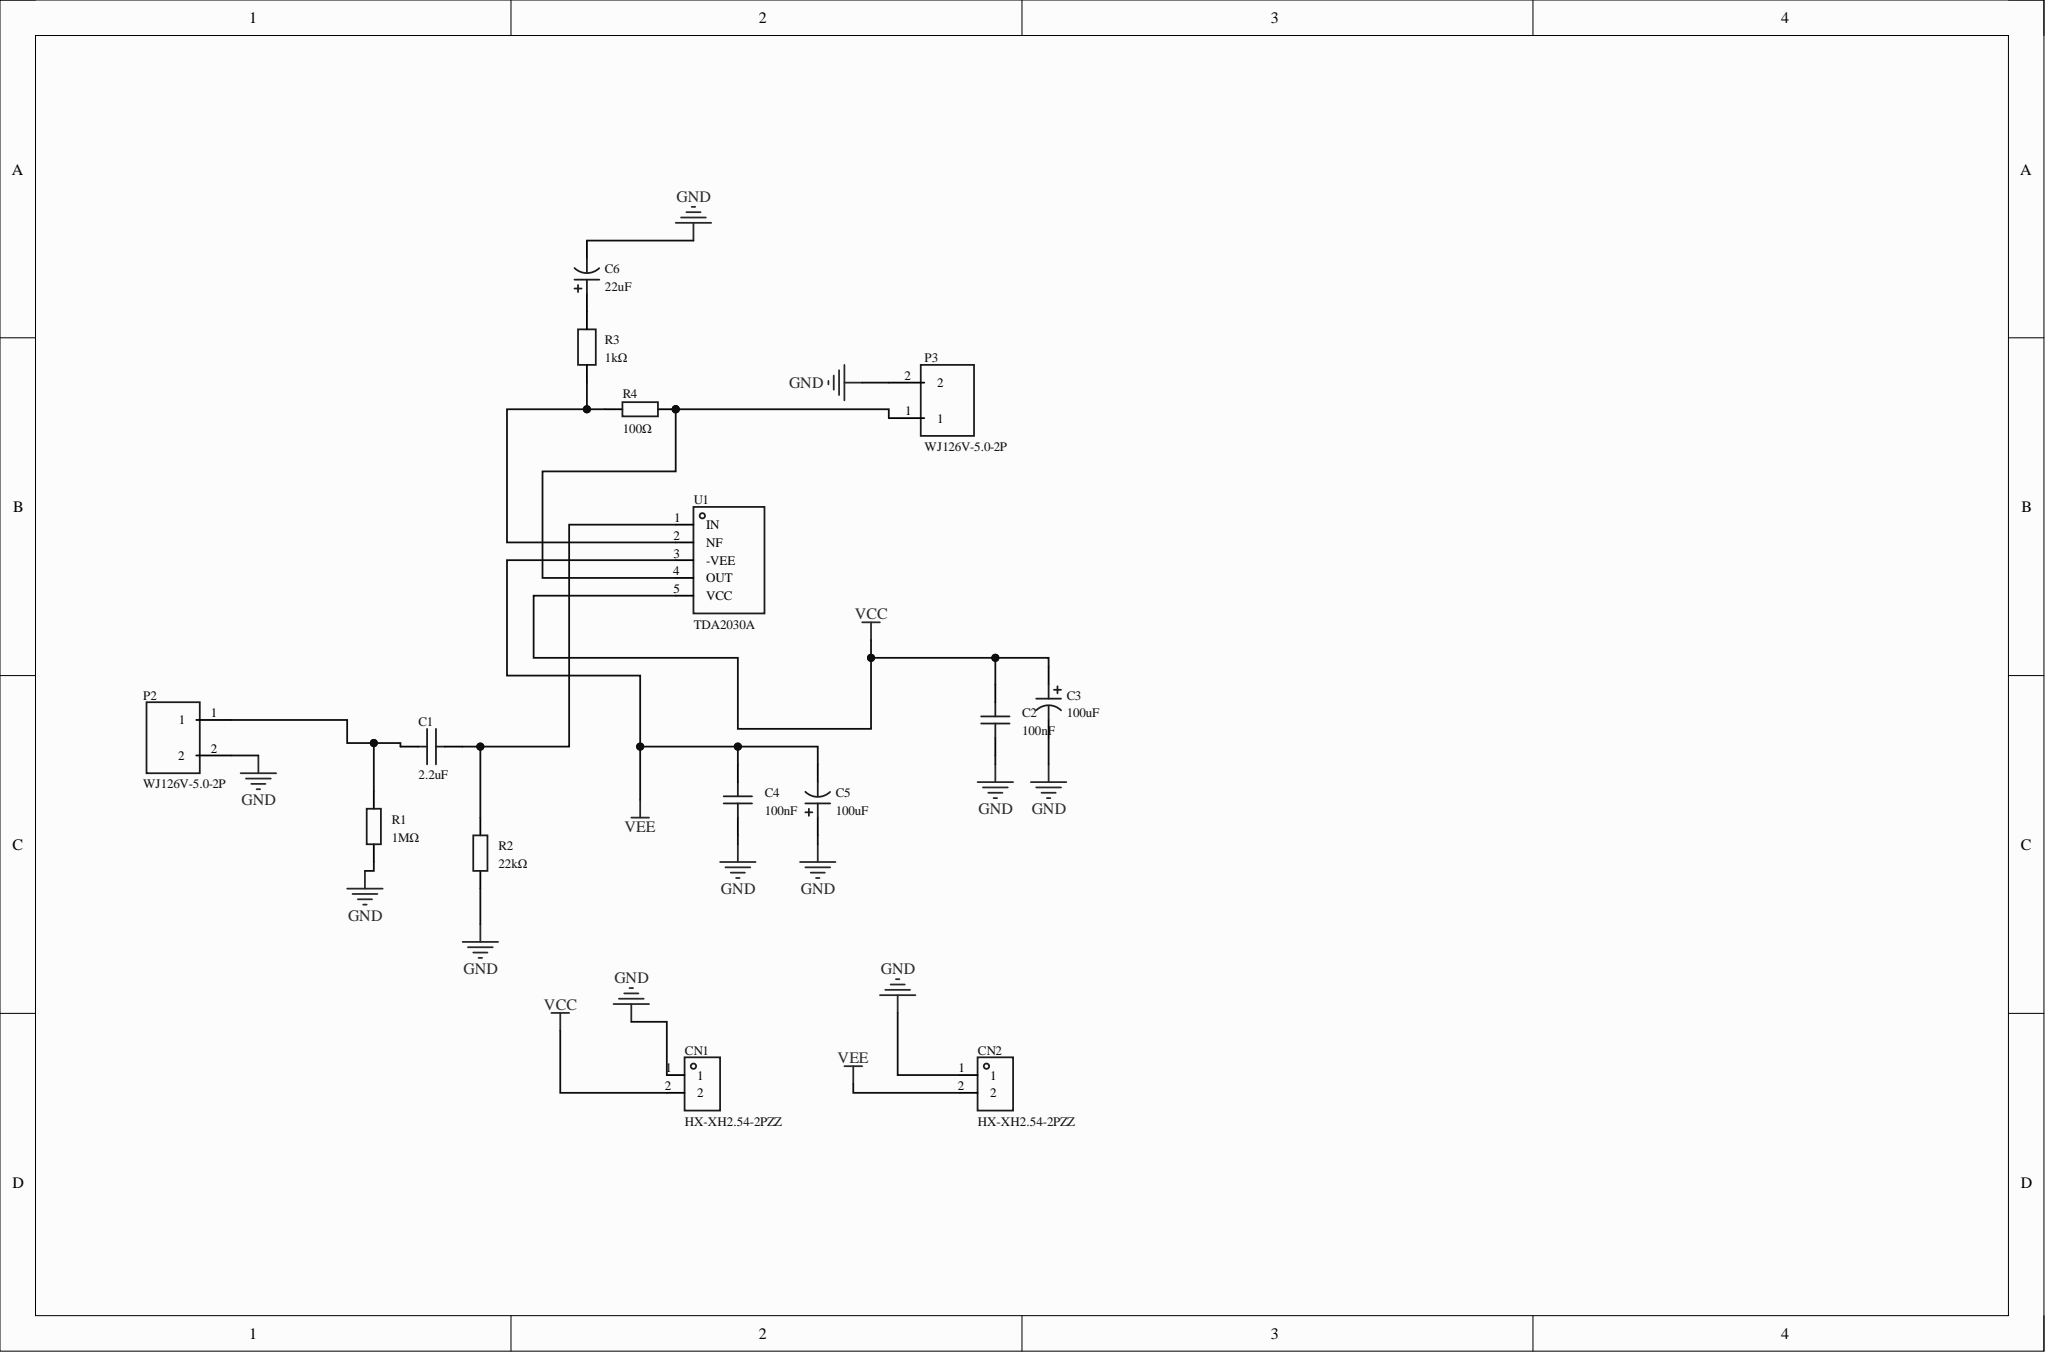Circuit board | Altium Designer | 15 parts | 8 nets
Bill of materials:
Comment,Description,Designator,Footprint,LibRef,Quantity
"2.2uF","Capacitance:2.2uF;Tolerance:±20%;Rated voltage:6.3V;Temperature coefficient:X5R;","C1","C0402","CL05A225MQ5NSNC","1"
"100nF","Capacitance:100nF;Tolerance:±10%;Rated voltage:50V;Temperature coefficient:X7R;","C2, C4","C0603","CGA0603X7R104K500JT","2"
"100uF","Capacitance:100uF;Tolerance:±20%;Rated voltage:50V;Ripple current:680mA@100kHz;Equivalent series resistance(ESR):120mΩ@100kHz;","C3, C5","CAP-TH_BD8.0-P3.50-D0.5-FD","ERG50V100M8X12","2"
"22uF","Capacitance:22uF;Tolerance:±20%;Rated voltage:400V;Ripple current:145mA@100kHz;Equivalent series resistance(ESR):7.8Ω@100kHz;","C6","CAP-TH_BD10.0-P5.00-D0.6-FD","ERG400V22M10X17","1"
"HX-XH2.54-2PZZ","Pin structure:1x2P;Pitch:2.54mm;Mounting:through-hole;Reference series:XH;Total pins:2P;Rows:1;Pins per row:2;Row spacing:-;Rated current:3A;Contact material:brass;Contact plating:tin;Working temperature:-25℃~+85℃;","CN1, CN2","CONN-TH_2P-P2.50_HX-2.54MM-2P-ZZ-MS","HX-XH2.54-2PZZ","2"
"WJ126V-5.0-2P","Structure:1x2P;Pitch:5mm;Colour:green;Mounting:through-hole;Rows:1;Pins per row:2;Rated current:18A;Rated voltage:250V;Wire gauge - AWG:14~26;Wire gauge - sq mm:2.5;Working temperature:-40℃~+105℃;","P2, P3","CONN-TH_WJ126V-5.0-2P","WJ126V-5.0-2P","2"
"1MΩ","Resistor type:thick film;Resistance:1MΩ;Tolerance:±1%;Power:100mW;Max working voltage:75V;Temperature coefficient:±100ppm/?;","R1","R0603","0603WAF1004T5E","1"
"22kΩ","Resistor type:thick film;Resistance:22kΩ;Tolerance:±1%;Power:100mW;Working voltage:75V;Temperature coefficient:±100ppm/?;","R2","R0603","0603WAF2202T5E","1"
"1kΩ","Resistor type:thick film;Resistance:1kΩ;Tolerance:±1%;Power:100mW;Working voltage:75V;Temperature coefficient:±100ppm/?;","R3","R0603","FRC0603F1001TS","1"
"100Ω","Resistor type:thick film;Resistance:100Ω;Tolerance:±1%;Power:125mW;Max working voltage:150V;Temperature coefficient:±100ppm/?;","R4","R0805","0805W8F1000T5E","1"
"TDA2030A","Amplifier type:-;Speaker channels:mono;Output power:18W;Quiescent current(Iq):40mA;","U1","TO-220B-5_L10.6-W8.7-P1.70-BL","TDA2030A","1"
Netlist (Protel format):
[
C1
C0402
2.2uF



]
[
C2
C0603
100nF



]
[
C3
CAP-TH_BD8.0-P3.50-D0.5-FD
100uF



]
[
C4
C0603
100nF



]
[
C5
CAP-TH_BD8.0-P3.50-D0.5-FD
100uF



]
[
C6
CAP-TH_BD10.0-P5.00-D0.6-FD
22uF



]
[
CN1
CONN-TH_2P-P2.50_HX-2.54MM-2P-ZZ-MS
HX-XH2.54-2PZZ



]
[
CN2
CONN-TH_2P-P2.50_HX-2.54MM-2P-ZZ-MS
HX-XH2.54-2PZZ



]
[
P2
CONN-TH_WJ126V-5.0-2P
WJ126V-5.0-2P



]
[
P3
CONN-TH_WJ126V-5.0-2P
WJ126V-5.0-2P



]
[
R1
R0603
1MΩ



]
[
R2
R0603
22kΩ



]
[
R3
R0603
1kΩ



]
[
R4
R0805
100Ω



]
[
U1
TO-220B-5_L10.6-W8.7-P1.70-BL
TDA2030A



]
(
VEE
C4-2
C5-2
CN2-2
U1-3
)
(
VCC
C2-2
C3-1
CN1-2
U1-5
)
(
NetR3_1
R3-1
R4-1
U1-2
)
(
NetP3_1
P3-1
R4-2
U1-4
)
(
NetC6_1
C6-1
R3-2
)
(
NetC1_2
C1-2
R2-2
U1-1
)
(
NetC1_1
C1-1
P2-1
R1-2
)
(
GND
C2-1
C3-2
C4-1
C5-1
C6-2
CN1-1
CN2-1
P2-2
P3-2
R1-1
R2-1
)